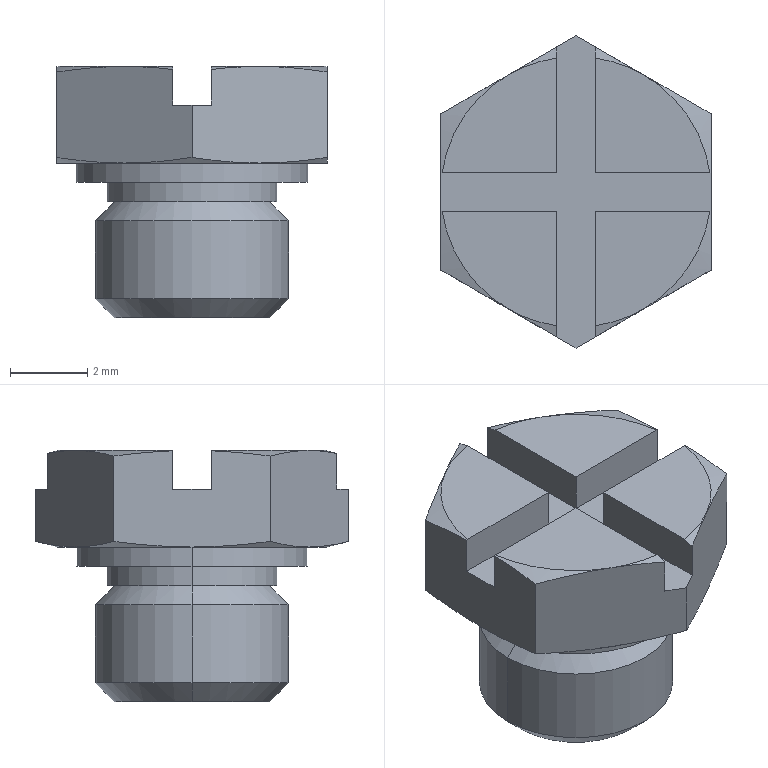Part | SolidWorks | features BaseBody 1 | 1 solid | 47 faces | box 7 x 8.083 x 6.5 mm | volume 169.1 mm3 | plane 23 | cone 18 | cylinder 6 | commonest cylinder face diameters 4.4 x2 5 x2 6 x2
STEP:
#1=CARTESIAN_POINT('',(2.5,0.,-3.01));
#2=VERTEX_POINT('',#1);
#3=CARTESIAN_POINT('',(-2.5,0.,-3.01));
#4=VERTEX_POINT('',#3);
#5=CARTESIAN_POINT('',(0.,0.,-3.01));
#6=DIRECTION('',(0.,0.,1.));
#7=DIRECTION('',(1.,0.,0.));
#8=AXIS2_PLACEMENT_3D('',#5,#6,#7);
#9=CIRCLE('',#8,2.5);
#10=EDGE_CURVE('',#2,#4,#9,.T.);
#11=ORIENTED_EDGE('',*,*,#10,.T.);
#12=CARTESIAN_POINT('',(-2.5,0.,-0.9905));
#13=VERTEX_POINT('',#12);
#14=CARTESIAN_POINT('',(-2.5,0.,-3.5));
#15=DIRECTION('',(0.,0.,1.));
#16=VECTOR('',#15,1000.);
#17=LINE('',#14,#16);
#18=EDGE_CURVE('',#4,#13,#17,.T.);
#19=ORIENTED_EDGE('',*,*,#18,.T.);
#20=CARTESIAN_POINT('',(2.5,0.,-0.9905));
#21=VERTEX_POINT('',#20);
#22=CARTESIAN_POINT('',(0.,0.,-0.9905));
#23=DIRECTION('',(0.,0.,-1.));
#24=DIRECTION('',(1.,0.,0.));
#25=AXIS2_PLACEMENT_3D('',#22,#23,#24);
#26=CIRCLE('',#25,2.5);
#27=EDGE_CURVE('',#13,#21,#26,.T.);
#28=ORIENTED_EDGE('',*,*,#27,.T.);
#29=CARTESIAN_POINT('',(2.5,0.,-3.5));
#30=DIRECTION('',(0.,0.,1.));
#31=VECTOR('',#30,1000.);
#32=LINE('',#29,#31);
#33=EDGE_CURVE('',#2,#21,#32,.T.);
#34=ORIENTED_EDGE('',*,*,#33,.F.);
#35=EDGE_LOOP('',(#11,#19,#28,#34));
#36=FACE_OUTER_BOUND('',#35,.T.);
#37=CARTESIAN_POINT('',(0.,0.,-3.5));
#38=DIRECTION('',(0.,0.,1.));
#39=DIRECTION('',(1.,0.,0.));
#40=AXIS2_PLACEMENT_3D('',#37,#38,#39);
#41=CYLINDRICAL_SURFACE('',#40,2.5);
#42=ADVANCED_FACE('',(#36),#41,.T.);
#43=CARTESIAN_POINT('',(-2.009,0.,-0.5));
#44=VERTEX_POINT('',#43);
#45=CARTESIAN_POINT('',(2.009,0.,-0.5));
#46=VERTEX_POINT('',#45);
#47=CARTESIAN_POINT('',(0.,0.,-0.5));
#48=DIRECTION('',(0.,0.,-1.));
#49=DIRECTION('',(-1.,0.,0.));
#50=AXIS2_PLACEMENT_3D('',#47,#48,#49);
#51=CIRCLE('',#50,2.009);
#52=EDGE_CURVE('',#44,#46,#51,.T.);
#53=ORIENTED_EDGE('',*,*,#52,.T.);
#54=CARTESIAN_POINT('',(2.5,0.,-0.9905));
#55=DIRECTION('',(0.7071,0.,-0.7071));
#56=VECTOR('',#55,1000.);
#57=LINE('',#54,#56);
#58=EDGE_CURVE('',#46,#21,#57,.T.);
#59=ORIENTED_EDGE('',*,*,#58,.T.);
#60=ORIENTED_EDGE('',*,*,#27,.F.);
#61=CARTESIAN_POINT('',(-2.5,0.,-0.9905));
#62=DIRECTION('',(-0.7071,0.,-0.7071));
#63=VECTOR('',#62,1000.);
#64=LINE('',#61,#63);
#65=EDGE_CURVE('',#44,#13,#64,.T.);
#66=ORIENTED_EDGE('',*,*,#65,.F.);
#67=EDGE_LOOP('',(#53,#59,#60,#66));
#68=FACE_OUTER_BOUND('',#67,.T.);
#69=CARTESIAN_POINT('',(0.,0.,-0.9905));
#70=DIRECTION('',(0.,0.,-1.));
#71=DIRECTION('',(-1.,0.,0.));
#72=AXIS2_PLACEMENT_3D('',#69,#70,#71);
#73=CONICAL_SURFACE('',#72,2.5,0.7854);
#74=ADVANCED_FACE('',(#68),#73,.T.);
#75=CARTESIAN_POINT('',(2.009,0.,-3.5));
#76=VERTEX_POINT('',#75);
#77=CARTESIAN_POINT('',(-2.009,0.,-3.5));
#78=VERTEX_POINT('',#77);
#79=CARTESIAN_POINT('',(0.,0.,-3.5));
#80=DIRECTION('',(0.,0.,1.));
#81=DIRECTION('',(1.,0.,0.));
#82=AXIS2_PLACEMENT_3D('',#79,#80,#81);
#83=CIRCLE('',#82,2.009);
#84=EDGE_CURVE('',#76,#78,#83,.T.);
#85=ORIENTED_EDGE('',*,*,#84,.T.);
#86=CARTESIAN_POINT('',(-2.5,0.,-3.01));
#87=DIRECTION('',(-0.7071,0.,0.7071));
#88=VECTOR('',#87,1000.);
#89=LINE('',#86,#88);
#90=EDGE_CURVE('',#78,#4,#89,.T.);
#91=ORIENTED_EDGE('',*,*,#90,.T.);
#92=ORIENTED_EDGE('',*,*,#10,.F.);
#93=CARTESIAN_POINT('',(2.5,0.,-3.01));
#94=DIRECTION('',(0.7071,0.,0.7071));
#95=VECTOR('',#94,1000.);
#96=LINE('',#93,#95);
#97=EDGE_CURVE('',#76,#2,#96,.T.);
#98=ORIENTED_EDGE('',*,*,#97,.F.);
#99=EDGE_LOOP('',(#85,#91,#92,#98));
#100=FACE_OUTER_BOUND('',#99,.T.);
#101=CARTESIAN_POINT('',(0.,0.,-3.01));
#102=DIRECTION('',(0.,0.,1.));
#103=DIRECTION('',(1.,0.,0.));
#104=AXIS2_PLACEMENT_3D('',#101,#102,#103);
#105=CONICAL_SURFACE('',#104,2.5,0.7854);
#106=ADVANCED_FACE('',(#100),#105,.T.);
#107=CARTESIAN_POINT('',(2.2,0.,-0.5));
#108=VERTEX_POINT('',#107);
#109=CARTESIAN_POINT('',(-2.2,0.,-0.5));
#110=VERTEX_POINT('',#109);
#111=CARTESIAN_POINT('',(0.,0.,-0.5));
#112=DIRECTION('',(0.,0.,1.));
#113=DIRECTION('',(1.,0.,0.));
#114=AXIS2_PLACEMENT_3D('',#111,#112,#113);
#115=CIRCLE('',#114,2.2);
#116=EDGE_CURVE('',#108,#110,#115,.T.);
#117=ORIENTED_EDGE('',*,*,#116,.T.);
#118=CARTESIAN_POINT('',(-2.2,0.,0.));
#119=VERTEX_POINT('',#118);
#120=CARTESIAN_POINT('',(-2.2,0.,-3.5));
#121=DIRECTION('',(0.,0.,1.));
#122=VECTOR('',#121,1000.);
#123=LINE('',#120,#122);
#124=EDGE_CURVE('',#110,#119,#123,.T.);
#125=ORIENTED_EDGE('',*,*,#124,.T.);
#126=CARTESIAN_POINT('',(2.2,0.,0.));
#127=VERTEX_POINT('',#126);
#128=CARTESIAN_POINT('',(0.,0.,0.));
#129=DIRECTION('',(0.,0.,-1.));
#130=DIRECTION('',(1.,0.,0.));
#131=AXIS2_PLACEMENT_3D('',#128,#129,#130);
#132=CIRCLE('',#131,2.2);
#133=EDGE_CURVE('',#119,#127,#132,.T.);
#134=ORIENTED_EDGE('',*,*,#133,.T.);
#135=CARTESIAN_POINT('',(2.2,0.,-3.5));
#136=DIRECTION('',(0.,0.,1.));
#137=VECTOR('',#136,1000.);
#138=LINE('',#135,#137);
#139=EDGE_CURVE('',#108,#127,#138,.T.);
#140=ORIENTED_EDGE('',*,*,#139,.F.);
#141=EDGE_LOOP('',(#117,#125,#134,#140));
#142=FACE_OUTER_BOUND('',#141,.T.);
#143=CARTESIAN_POINT('',(0.,0.,-3.5));
#144=DIRECTION('',(0.,0.,1.));
#145=DIRECTION('',(1.,0.,0.));
#146=AXIS2_PLACEMENT_3D('',#143,#144,#145);
#147=CYLINDRICAL_SURFACE('',#146,2.2);
#148=ADVANCED_FACE('',(#142),#147,.T.);
#149=CARTESIAN_POINT('',(3.,0.,0.));
#150=VERTEX_POINT('',#149);
#151=CARTESIAN_POINT('',(-3.,0.,0.));
#152=VERTEX_POINT('',#151);
#153=CARTESIAN_POINT('',(0.,0.,0.));
#154=DIRECTION('',(0.,0.,1.));
#155=DIRECTION('',(1.,0.,0.));
#156=AXIS2_PLACEMENT_3D('',#153,#154,#155);
#157=CIRCLE('',#156,3.);
#158=EDGE_CURVE('',#150,#152,#157,.T.);
#159=ORIENTED_EDGE('',*,*,#158,.T.);
#160=CARTESIAN_POINT('',(-3.,0.,0.5));
#161=VERTEX_POINT('',#160);
#162=CARTESIAN_POINT('',(-3.,0.,-3.5));
#163=DIRECTION('',(0.,0.,1.));
#164=VECTOR('',#163,1000.);
#165=LINE('',#162,#164);
#166=EDGE_CURVE('',#152,#161,#165,.T.);
#167=ORIENTED_EDGE('',*,*,#166,.T.);
#168=CARTESIAN_POINT('',(3.,0.,0.5));
#169=VERTEX_POINT('',#168);
#170=CARTESIAN_POINT('',(0.,0.,0.5));
#171=DIRECTION('',(0.,0.,-1.));
#172=DIRECTION('',(1.,0.,0.));
#173=AXIS2_PLACEMENT_3D('',#170,#171,#172);
#174=CIRCLE('',#173,3.);
#175=EDGE_CURVE('',#161,#169,#174,.T.);
#176=ORIENTED_EDGE('',*,*,#175,.T.);
#177=CARTESIAN_POINT('',(3.,0.,-3.5));
#178=DIRECTION('',(0.,0.,1.));
#179=VECTOR('',#178,1000.);
#180=LINE('',#177,#179);
#181=EDGE_CURVE('',#150,#169,#180,.T.);
#182=ORIENTED_EDGE('',*,*,#181,.F.);
#183=EDGE_LOOP('',(#159,#167,#176,#182));
#184=FACE_OUTER_BOUND('',#183,.T.);
#185=CARTESIAN_POINT('',(0.,0.,-3.5));
#186=DIRECTION('',(0.,0.,1.));
#187=DIRECTION('',(1.,0.,0.));
#188=AXIS2_PLACEMENT_3D('',#185,#186,#187);
#189=CYLINDRICAL_SURFACE('',#188,3.);
#190=ADVANCED_FACE('',(#184),#189,.T.);
#191=ORIENTED_EDGE('',*,*,#18,.F.);
#192=CARTESIAN_POINT('',(0.,0.,-3.01));
#193=DIRECTION('',(0.,0.,1.));
#194=DIRECTION('',(1.,0.,0.));
#195=AXIS2_PLACEMENT_3D('',#192,#193,#194);
#196=CIRCLE('',#195,2.5);
#197=EDGE_CURVE('',#4,#2,#196,.T.);
#198=ORIENTED_EDGE('',*,*,#197,.T.);
#199=ORIENTED_EDGE('',*,*,#33,.T.);
#200=CARTESIAN_POINT('',(0.,0.,-0.9905));
#201=DIRECTION('',(0.,0.,-1.));
#202=DIRECTION('',(1.,0.,0.));
#203=AXIS2_PLACEMENT_3D('',#200,#201,#202);
#204=CIRCLE('',#203,2.5);
#205=EDGE_CURVE('',#21,#13,#204,.T.);
#206=ORIENTED_EDGE('',*,*,#205,.T.);
#207=EDGE_LOOP('',(#191,#198,#199,#206));
#208=FACE_OUTER_BOUND('',#207,.T.);
#209=CARTESIAN_POINT('',(0.,0.,-3.5));
#210=DIRECTION('',(0.,0.,1.));
#211=DIRECTION('',(1.,0.,0.));
#212=AXIS2_PLACEMENT_3D('',#209,#210,#211);
#213=CYLINDRICAL_SURFACE('',#212,2.5);
#214=ADVANCED_FACE('',(#208),#213,.T.);
#215=ORIENTED_EDGE('',*,*,#58,.F.);
#216=CARTESIAN_POINT('',(0.,0.,-0.5));
#217=DIRECTION('',(0.,0.,-1.));
#218=DIRECTION('',(-1.,0.,0.));
#219=AXIS2_PLACEMENT_3D('',#216,#217,#218);
#220=CIRCLE('',#219,2.009);
#221=EDGE_CURVE('',#46,#44,#220,.T.);
#222=ORIENTED_EDGE('',*,*,#221,.T.);
#223=ORIENTED_EDGE('',*,*,#65,.T.);
#224=ORIENTED_EDGE('',*,*,#205,.F.);
#225=EDGE_LOOP('',(#215,#222,#223,#224));
#226=FACE_OUTER_BOUND('',#225,.T.);
#227=CARTESIAN_POINT('',(0.,0.,-0.9905));
#228=DIRECTION('',(0.,0.,-1.));
#229=DIRECTION('',(-1.,0.,0.));
#230=AXIS2_PLACEMENT_3D('',#227,#228,#229);
#231=CONICAL_SURFACE('',#230,2.5,0.7854);
#232=ADVANCED_FACE('',(#226),#231,.T.);
#233=ORIENTED_EDGE('',*,*,#90,.F.);
#234=CARTESIAN_POINT('',(0.,0.,-3.5));
#235=DIRECTION('',(0.,0.,1.));
#236=DIRECTION('',(1.,0.,0.));
#237=AXIS2_PLACEMENT_3D('',#234,#235,#236);
#238=CIRCLE('',#237,2.009);
#239=EDGE_CURVE('',#78,#76,#238,.T.);
#240=ORIENTED_EDGE('',*,*,#239,.T.);
#241=ORIENTED_EDGE('',*,*,#97,.T.);
#242=ORIENTED_EDGE('',*,*,#197,.F.);
#243=EDGE_LOOP('',(#233,#240,#241,#242));
#244=FACE_OUTER_BOUND('',#243,.T.);
#245=CARTESIAN_POINT('',(0.,0.,-3.01));
#246=DIRECTION('',(0.,0.,1.));
#247=DIRECTION('',(1.,0.,0.));
#248=AXIS2_PLACEMENT_3D('',#245,#246,#247);
#249=CONICAL_SURFACE('',#248,2.5,0.7854);
#250=ADVANCED_FACE('',(#244),#249,.T.);
#251=ORIENTED_EDGE('',*,*,#52,.F.);
#252=ORIENTED_EDGE('',*,*,#221,.F.);
#253=EDGE_LOOP('',(#251,#252));
#254=FACE_BOUND('',#253,.T.);
#255=ORIENTED_EDGE('',*,*,#116,.F.);
#256=CARTESIAN_POINT('',(0.,0.,-0.5));
#257=DIRECTION('',(0.,0.,1.));
#258=DIRECTION('',(1.,0.,0.));
#259=AXIS2_PLACEMENT_3D('',#256,#257,#258);
#260=CIRCLE('',#259,2.2);
#261=EDGE_CURVE('',#110,#108,#260,.T.);
#262=ORIENTED_EDGE('',*,*,#261,.F.);
#263=EDGE_LOOP('',(#255,#262));
#264=FACE_OUTER_BOUND('',#263,.T.);
#265=CARTESIAN_POINT('',(0.,2.2,-0.5));
#266=DIRECTION('',(0.,0.,1.));
#267=DIRECTION('',(1.,0.,0.));
#268=AXIS2_PLACEMENT_3D('',#265,#266,#267);
#269=PLANE('',#268);
#270=ADVANCED_FACE('',(#254,#264),#269,.F.);
#271=ORIENTED_EDGE('',*,*,#84,.F.);
#272=ORIENTED_EDGE('',*,*,#239,.F.);
#273=EDGE_LOOP('',(#271,#272));
#274=FACE_OUTER_BOUND('',#273,.T.);
#275=CARTESIAN_POINT('',(0.,2.01,-3.5));
#276=DIRECTION('',(0.,0.,1.));
#277=DIRECTION('',(1.,0.,0.));
#278=AXIS2_PLACEMENT_3D('',#275,#276,#277);
#279=PLANE('',#278);
#280=ADVANCED_FACE('',(#274),#279,.F.);
#281=ORIENTED_EDGE('',*,*,#124,.F.);
#282=ORIENTED_EDGE('',*,*,#261,.T.);
#283=ORIENTED_EDGE('',*,*,#139,.T.);
#284=CARTESIAN_POINT('',(0.,0.,0.));
#285=DIRECTION('',(0.,0.,-1.));
#286=DIRECTION('',(1.,0.,0.));
#287=AXIS2_PLACEMENT_3D('',#284,#285,#286);
#288=CIRCLE('',#287,2.2);
#289=EDGE_CURVE('',#127,#119,#288,.T.);
#290=ORIENTED_EDGE('',*,*,#289,.T.);
#291=EDGE_LOOP('',(#281,#282,#283,#290));
#292=FACE_OUTER_BOUND('',#291,.T.);
#293=CARTESIAN_POINT('',(0.,0.,-3.5));
#294=DIRECTION('',(0.,0.,1.));
#295=DIRECTION('',(1.,0.,0.));
#296=AXIS2_PLACEMENT_3D('',#293,#294,#295);
#297=CYLINDRICAL_SURFACE('',#296,2.2);
#298=ADVANCED_FACE('',(#292),#297,.T.);
#299=ORIENTED_EDGE('',*,*,#289,.F.);
#300=ORIENTED_EDGE('',*,*,#133,.F.);
#301=EDGE_LOOP('',(#299,#300));
#302=FACE_BOUND('',#301,.T.);
#303=ORIENTED_EDGE('',*,*,#158,.F.);
#304=CARTESIAN_POINT('',(0.,0.,0.));
#305=DIRECTION('',(0.,0.,1.));
#306=DIRECTION('',(1.,0.,0.));
#307=AXIS2_PLACEMENT_3D('',#304,#305,#306);
#308=CIRCLE('',#307,3.);
#309=EDGE_CURVE('',#152,#150,#308,.T.);
#310=ORIENTED_EDGE('',*,*,#309,.F.);
#311=EDGE_LOOP('',(#303,#310));
#312=FACE_OUTER_BOUND('',#311,.T.);
#313=CARTESIAN_POINT('',(0.,3.,0.));
#314=DIRECTION('',(0.,0.,1.));
#315=DIRECTION('',(1.,0.,0.));
#316=AXIS2_PLACEMENT_3D('',#313,#314,#315);
#317=PLANE('',#316);
#318=ADVANCED_FACE('',(#302,#312),#317,.F.);
#319=ORIENTED_EDGE('',*,*,#166,.F.);
#320=ORIENTED_EDGE('',*,*,#309,.T.);
#321=ORIENTED_EDGE('',*,*,#181,.T.);
#322=CARTESIAN_POINT('',(0.,0.,0.5));
#323=DIRECTION('',(0.,0.,-1.));
#324=DIRECTION('',(1.,0.,0.));
#325=AXIS2_PLACEMENT_3D('',#322,#323,#324);
#326=CIRCLE('',#325,3.);
#327=EDGE_CURVE('',#169,#161,#326,.T.);
#328=ORIENTED_EDGE('',*,*,#327,.T.);
#329=EDGE_LOOP('',(#319,#320,#321,#328));
#330=FACE_OUTER_BOUND('',#329,.T.);
#331=CARTESIAN_POINT('',(0.,0.,-3.5));
#332=DIRECTION('',(0.,0.,1.));
#333=DIRECTION('',(1.,0.,0.));
#334=AXIS2_PLACEMENT_3D('',#331,#332,#333);
#335=CYLINDRICAL_SURFACE('',#334,3.);
#336=ADVANCED_FACE('',(#330),#335,.T.);
#337=ORIENTED_EDGE('',*,*,#327,.F.);
#338=ORIENTED_EDGE('',*,*,#175,.F.);
#339=EDGE_LOOP('',(#337,#338));
#340=FACE_BOUND('',#339,.T.);
#341=CARTESIAN_POINT('',(3.5,0.,0.5));
#342=VERTEX_POINT('',#341);
#343=CARTESIAN_POINT('',(1.75,3.031,0.5));
#344=VERTEX_POINT('',#343);
#345=CARTESIAN_POINT('',(0.,0.,0.5));
#346=DIRECTION('',(0.,0.,1.));
#347=DIRECTION('',(1.,0.,0.));
#348=AXIS2_PLACEMENT_3D('',#345,#346,#347);
#349=CIRCLE('',#348,3.5);
#350=EDGE_CURVE('',#342,#344,#349,.T.);
#351=ORIENTED_EDGE('',*,*,#350,.F.);
#352=CARTESIAN_POINT('',(1.75,-3.031,0.5));
#353=VERTEX_POINT('',#352);
#354=CARTESIAN_POINT('',(0.,0.,0.5));
#355=DIRECTION('',(0.,0.,1.));
#356=DIRECTION('',(1.,0.,0.));
#357=AXIS2_PLACEMENT_3D('',#354,#355,#356);
#358=CIRCLE('',#357,3.5);
#359=EDGE_CURVE('',#353,#342,#358,.T.);
#360=ORIENTED_EDGE('',*,*,#359,.F.);
#361=CARTESIAN_POINT('',(-1.75,-3.031,0.5));
#362=VERTEX_POINT('',#361);
#363=CARTESIAN_POINT('',(0.,0.,0.5));
#364=DIRECTION('',(0.,0.,1.));
#365=DIRECTION('',(1.,0.,0.));
#366=AXIS2_PLACEMENT_3D('',#363,#364,#365);
#367=CIRCLE('',#366,3.5);
#368=EDGE_CURVE('',#362,#353,#367,.T.);
#369=ORIENTED_EDGE('',*,*,#368,.F.);
#370=CARTESIAN_POINT('',(-3.5,0.,0.5));
#371=VERTEX_POINT('',#370);
#372=CARTESIAN_POINT('',(0.,0.,0.5));
#373=DIRECTION('',(0.,0.,1.));
#374=DIRECTION('',(1.,0.,0.));
#375=AXIS2_PLACEMENT_3D('',#372,#373,#374);
#376=CIRCLE('',#375,3.5);
#377=EDGE_CURVE('',#371,#362,#376,.T.);
#378=ORIENTED_EDGE('',*,*,#377,.F.);
#379=CARTESIAN_POINT('',(-1.75,3.031,0.5));
#380=VERTEX_POINT('',#379);
#381=CARTESIAN_POINT('',(0.,0.,0.5));
#382=DIRECTION('',(0.,0.,1.));
#383=DIRECTION('',(1.,0.,0.));
#384=AXIS2_PLACEMENT_3D('',#381,#382,#383);
#385=CIRCLE('',#384,3.5);
#386=EDGE_CURVE('',#380,#371,#385,.T.);
#387=ORIENTED_EDGE('',*,*,#386,.F.);
#388=CARTESIAN_POINT('',(0.,0.,0.5));
#389=DIRECTION('',(0.,0.,1.));
#390=DIRECTION('',(1.,0.,0.));
#391=AXIS2_PLACEMENT_3D('',#388,#389,#390);
#392=CIRCLE('',#391,3.5);
#393=EDGE_CURVE('',#344,#380,#392,.T.);
#394=ORIENTED_EDGE('',*,*,#393,.F.);
#395=EDGE_LOOP('',(#351,#360,#369,#378,#387,#394));
#396=FACE_OUTER_BOUND('',#395,.T.);
#397=CARTESIAN_POINT('',(0.,3.5,0.5));
#398=DIRECTION('',(0.,0.,1.));
#399=DIRECTION('',(1.,0.,0.));
#400=AXIS2_PLACEMENT_3D('',#397,#398,#399);
#401=PLANE('',#400);
#402=ADVANCED_FACE('',(#340,#396),#401,.F.);
#403=CARTESIAN_POINT('',(-0.000000057,4.041,0.6451));
#404=VERTEX_POINT('',#403);
#405=CARTESIAN_POINT('',(-0.000000057,4.041,0.6451));
#406=CARTESIAN_POINT('',(0.5808,3.706,0.5552));
#407=CARTESIAN_POINT('',(1.164,3.37,0.5));
#408=CARTESIAN_POINT('',(1.75,3.031,0.5));
#409=B_SPLINE_CURVE_WITH_KNOTS('',3,(#405,#406,#407,#408),.UNSPECIFIED.,.F.,.F.,(4,4),(0.,0.002026),.UNSPECIFIED.);
#410=EDGE_CURVE('',#404,#344,#409,.T.);
#411=ORIENTED_EDGE('',*,*,#410,.T.);
#412=ORIENTED_EDGE('',*,*,#393,.T.);
#413=CARTESIAN_POINT('',(-1.75,3.031,0.5));
#414=CARTESIAN_POINT('',(-1.164,3.37,0.5));
#415=CARTESIAN_POINT('',(-0.5808,3.706,0.5552));
#416=CARTESIAN_POINT('',(-0.000000057,4.041,0.6451));
#417=B_SPLINE_CURVE_WITH_KNOTS('',3,(#413,#414,#415,#416),.UNSPECIFIED.,.F.,.F.,(4,4),(0.,0.002026),.UNSPECIFIED.);
#418=EDGE_CURVE('',#380,#404,#417,.T.);
#419=ORIENTED_EDGE('',*,*,#418,.T.);
#420=EDGE_LOOP('',(#411,#412,#419));
#421=FACE_OUTER_BOUND('',#420,.T.);
#422=CARTESIAN_POINT('',(0.,0.,0.646));
#423=DIRECTION('',(0.,0.,1.));
#424=DIRECTION('',(1.,0.,0.));
#425=AXIS2_PLACEMENT_3D('',#422,#423,#424);
#426=CONICAL_SURFACE('',#425,4.045,1.309);
#427=ADVANCED_FACE('',(#421),#426,.T.);
#428=CARTESIAN_POINT('',(3.5,2.021,0.6451));
#429=VERTEX_POINT('',#428);
#430=CARTESIAN_POINT('',(3.5,2.021,0.6451));
#431=CARTESIAN_POINT('',(3.5,1.35,0.5552));
#432=CARTESIAN_POINT('',(3.5,0.677,0.5));
#433=CARTESIAN_POINT('',(3.5,0.,0.5));
#434=B_SPLINE_CURVE_WITH_KNOTS('',3,(#430,#431,#432,#433),.UNSPECIFIED.,.F.,.F.,(4,4),(0.,0.002026),.UNSPECIFIED.);
#435=EDGE_CURVE('',#429,#342,#434,.T.);
#436=ORIENTED_EDGE('',*,*,#435,.T.);
#437=ORIENTED_EDGE('',*,*,#350,.T.);
#438=CARTESIAN_POINT('',(1.75,3.031,0.5));
#439=CARTESIAN_POINT('',(2.336,2.693,0.5));
#440=CARTESIAN_POINT('',(2.919,2.356,0.5552));
#441=CARTESIAN_POINT('',(3.5,2.021,0.6451));
#442=B_SPLINE_CURVE_WITH_KNOTS('',3,(#438,#439,#440,#441),.UNSPECIFIED.,.F.,.F.,(4,4),(0.,0.002026),.UNSPECIFIED.);
#443=EDGE_CURVE('',#344,#429,#442,.T.);
#444=ORIENTED_EDGE('',*,*,#443,.T.);
#445=EDGE_LOOP('',(#436,#437,#444));
#446=FACE_OUTER_BOUND('',#445,.T.);
#447=CARTESIAN_POINT('',(0.,0.,0.646));
#448=DIRECTION('',(0.,0.,1.));
#449=DIRECTION('',(1.,0.,0.));
#450=AXIS2_PLACEMENT_3D('',#447,#448,#449);
#451=CONICAL_SURFACE('',#450,4.045,1.309);
#452=ADVANCED_FACE('',(#446),#451,.T.);
#453=CARTESIAN_POINT('',(3.5,-2.021,0.6451));
#454=VERTEX_POINT('',#453);
#455=CARTESIAN_POINT('',(3.5,-2.021,0.6451));
#456=CARTESIAN_POINT('',(2.919,-2.356,0.5552));
#457=CARTESIAN_POINT('',(2.336,-2.693,0.5));
#458=CARTESIAN_POINT('',(1.75,-3.031,0.5));
#459=B_SPLINE_CURVE_WITH_KNOTS('',3,(#455,#456,#457,#458),.UNSPECIFIED.,.F.,.F.,(4,4),(0.,0.002026),.UNSPECIFIED.);
#460=EDGE_CURVE('',#454,#353,#459,.T.);
#461=ORIENTED_EDGE('',*,*,#460,.T.);
#462=ORIENTED_EDGE('',*,*,#359,.T.);
#463=CARTESIAN_POINT('',(3.5,0.,0.5));
#464=CARTESIAN_POINT('',(3.5,-0.677,0.5));
#465=CARTESIAN_POINT('',(3.5,-1.35,0.5552));
#466=CARTESIAN_POINT('',(3.5,-2.021,0.6451));
#467=B_SPLINE_CURVE_WITH_KNOTS('',3,(#463,#464,#465,#466),.UNSPECIFIED.,.F.,.F.,(4,4),(0.,0.002026),.UNSPECIFIED.);
#468=EDGE_CURVE('',#342,#454,#467,.T.);
#469=ORIENTED_EDGE('',*,*,#468,.T.);
#470=EDGE_LOOP('',(#461,#462,#469));
#471=FACE_OUTER_BOUND('',#470,.T.);
#472=CARTESIAN_POINT('',(0.,0.,0.646));
#473=DIRECTION('',(0.,0.,1.));
#474=DIRECTION('',(1.,0.,0.));
#475=AXIS2_PLACEMENT_3D('',#472,#473,#474);
#476=CONICAL_SURFACE('',#475,4.045,1.309);
#477=ADVANCED_FACE('',(#471),#476,.T.);
#478=CARTESIAN_POINT('',(0.000000064,-4.041,0.6451));
#479=VERTEX_POINT('',#478);
#480=CARTESIAN_POINT('',(0.000000064,-4.041,0.6451));
#481=CARTESIAN_POINT('',(-0.5808,-3.706,0.5552));
#482=CARTESIAN_POINT('',(-1.164,-3.37,0.5));
#483=CARTESIAN_POINT('',(-1.75,-3.031,0.5));
#484=B_SPLINE_CURVE_WITH_KNOTS('',3,(#480,#481,#482,#483),.UNSPECIFIED.,.F.,.F.,(4,4),(0.,0.002026),.UNSPECIFIED.);
#485=EDGE_CURVE('',#479,#362,#484,.T.);
#486=ORIENTED_EDGE('',*,*,#485,.T.);
#487=ORIENTED_EDGE('',*,*,#368,.T.);
#488=CARTESIAN_POINT('',(1.75,-3.031,0.5));
#489=CARTESIAN_POINT('',(1.164,-3.37,0.5));
#490=CARTESIAN_POINT('',(0.5808,-3.706,0.5552));
#491=CARTESIAN_POINT('',(0.000000064,-4.041,0.6451));
#492=B_SPLINE_CURVE_WITH_KNOTS('',3,(#488,#489,#490,#491),.UNSPECIFIED.,.F.,.F.,(4,4),(0.,0.002026),.UNSPECIFIED.);
#493=EDGE_CURVE('',#353,#479,#492,.T.);
#494=ORIENTED_EDGE('',*,*,#493,.T.);
#495=EDGE_LOOP('',(#486,#487,#494));
#496=FACE_OUTER_BOUND('',#495,.T.);
#497=CARTESIAN_POINT('',(0.,0.,0.646));
#498=DIRECTION('',(0.,0.,1.));
#499=DIRECTION('',(1.,0.,0.));
#500=AXIS2_PLACEMENT_3D('',#497,#498,#499);
#501=CONICAL_SURFACE('',#500,4.045,1.309);
#502=ADVANCED_FACE('',(#496),#501,.T.);
#503=ORIENTED_EDGE('',*,*,#377,.T.);
#504=CARTESIAN_POINT('',(-3.5,-2.021,0.6451));
#505=VERTEX_POINT('',#504);
#506=CARTESIAN_POINT('',(-1.75,-3.031,0.5));
#507=CARTESIAN_POINT('',(-2.336,-2.693,0.5));
#508=CARTESIAN_POINT('',(-2.919,-2.356,0.5552));
#509=CARTESIAN_POINT('',(-3.5,-2.021,0.6451));
#510=B_SPLINE_CURVE_WITH_KNOTS('',3,(#506,#507,#508,#509),.UNSPECIFIED.,.F.,.F.,(4,4),(0.,0.002026),.UNSPECIFIED.);
#511=EDGE_CURVE('',#362,#505,#510,.T.);
#512=ORIENTED_EDGE('',*,*,#511,.T.);
#513=CARTESIAN_POINT('',(-3.5,-2.021,0.6451));
#514=CARTESIAN_POINT('',(-3.5,-1.35,0.5552));
#515=CARTESIAN_POINT('',(-3.5,-0.677,0.5));
#516=CARTESIAN_POINT('',(-3.5,0.,0.5));
#517=B_SPLINE_CURVE_WITH_KNOTS('',3,(#513,#514,#515,#516),.UNSPECIFIED.,.F.,.F.,(4,4),(0.,0.002026),.UNSPECIFIED.);
#518=EDGE_CURVE('',#505,#371,#517,.T.);
#519=ORIENTED_EDGE('',*,*,#518,.T.);
#520=EDGE_LOOP('',(#503,#512,#519));
#521=FACE_OUTER_BOUND('',#520,.T.);
#522=CARTESIAN_POINT('',(0.,0.,0.646));
#523=DIRECTION('',(0.,0.,1.));
#524=DIRECTION('',(1.,0.,0.));
#525=AXIS2_PLACEMENT_3D('',#522,#523,#524);
#526=CONICAL_SURFACE('',#525,4.045,1.309);
#527=ADVANCED_FACE('',(#521),#526,.T.);
#528=CARTESIAN_POINT('',(-3.5,2.021,0.6451));
#529=VERTEX_POINT('',#528);
#530=CARTESIAN_POINT('',(-3.5,2.021,0.6451));
#531=CARTESIAN_POINT('',(-2.919,2.356,0.5552));
#532=CARTESIAN_POINT('',(-2.336,2.693,0.5));
#533=CARTESIAN_POINT('',(-1.75,3.031,0.5));
#534=B_SPLINE_CURVE_WITH_KNOTS('',3,(#530,#531,#532,#533),.UNSPECIFIED.,.F.,.F.,(4,4),(0.,0.002026),.UNSPECIFIED.);
#535=EDGE_CURVE('',#529,#380,#534,.T.);
#536=ORIENTED_EDGE('',*,*,#535,.T.);
#537=ORIENTED_EDGE('',*,*,#386,.T.);
#538=CARTESIAN_POINT('',(-3.5,0.,0.5));
#539=CARTESIAN_POINT('',(-3.5,0.677,0.5));
#540=CARTESIAN_POINT('',(-3.5,1.35,0.5552));
#541=CARTESIAN_POINT('',(-3.5,2.021,0.6451));
#542=B_SPLINE_CURVE_WITH_KNOTS('',3,(#538,#539,#540,#541),.UNSPECIFIED.,.F.,.F.,(4,4),(0.,0.002026),.UNSPECIFIED.);
#543=EDGE_CURVE('',#371,#529,#542,.T.);
#544=ORIENTED_EDGE('',*,*,#543,.T.);
#545=EDGE_LOOP('',(#536,#537,#544));
#546=FACE_OUTER_BOUND('',#545,.T.);
#547=CARTESIAN_POINT('',(0.,0.,0.646));
#548=DIRECTION('',(0.,0.,1.));
#549=DIRECTION('',(1.,0.,0.));
#550=AXIS2_PLACEMENT_3D('',#547,#548,#549);
#551=CONICAL_SURFACE('',#550,4.045,1.309);
#552=ADVANCED_FACE('',(#546),#551,.T.);
#553=CARTESIAN_POINT('',(1.75,3.031,3.));
#554=VERTEX_POINT('',#553);
#555=CARTESIAN_POINT('',(0.5,3.753,2.923));
#556=VERTEX_POINT('',#555);
#557=CARTESIAN_POINT('',(1.75,3.031,3.));
#558=CARTESIAN_POINT('',(1.332,3.272,3.));
#559=CARTESIAN_POINT('',(0.9156,3.513,2.972));
#560=CARTESIAN_POINT('',(0.5,3.753,2.923));
#561=B_SPLINE_CURVE_WITH_KNOTS('',3,(#557,#558,#559,#560),.UNSPECIFIED.,.F.,.F.,(4,4),(0.,0.001445),.UNSPECIFIED.);
#562=EDGE_CURVE('',#554,#556,#561,.T.);
#563=ORIENTED_EDGE('',*,*,#562,.F.);
#564=CARTESIAN_POINT('',(3.5,2.021,2.855));
#565=VERTEX_POINT('',#564);
#566=CARTESIAN_POINT('',(3.5,2.021,2.855));
#567=CARTESIAN_POINT('',(2.919,2.356,2.945));
#568=CARTESIAN_POINT('',(2.336,2.693,3.));
#569=CARTESIAN_POINT('',(1.75,3.031,3.));
#570=B_SPLINE_CURVE_WITH_KNOTS('',3,(#566,#567,#568,#569),.UNSPECIFIED.,.F.,.F.,(4,4),(0.,0.002026),.UNSPECIFIED.);
#571=EDGE_CURVE('',#565,#554,#570,.T.);
#572=ORIENTED_EDGE('',*,*,#571,.F.);
#573=CARTESIAN_POINT('',(3.5,2.021,3.));
#574=DIRECTION('',(0.,0.,1.));
#575=VECTOR('',#574,1000.);
#576=LINE('',#573,#575);
#577=EDGE_CURVE('',#429,#565,#576,.T.);
#578=ORIENTED_EDGE('',*,*,#577,.F.);
#579=ORIENTED_EDGE('',*,*,#443,.F.);
#580=ORIENTED_EDGE('',*,*,#410,.F.);
#581=CARTESIAN_POINT('',(0.,4.041,2.));
#582=VERTEX_POINT('',#581);
#583=CARTESIAN_POINT('',(0.,4.041,3.));
#584=DIRECTION('',(0.,0.,-1.));
#585=VECTOR('',#584,1000.);
#586=LINE('',#583,#585);
#587=EDGE_CURVE('',#582,#404,#586,.T.);
#588=ORIENTED_EDGE('',*,*,#587,.F.);
#589=CARTESIAN_POINT('',(0.5,3.753,2.));
#590=VERTEX_POINT('',#589);
#591=CARTESIAN_POINT('',(0.5,3.753,2.));
#592=DIRECTION('',(-0.866,0.5,0.));
#593=VECTOR('',#592,1000.);
#594=LINE('',#591,#593);
#595=EDGE_CURVE('',#590,#582,#594,.T.);
#596=ORIENTED_EDGE('',*,*,#595,.F.);
#597=CARTESIAN_POINT('',(0.5,3.753,2.));
#598=DIRECTION('',(0.,0.,1.));
#599=VECTOR('',#598,1000.);
#600=LINE('',#597,#599);
#601=EDGE_CURVE('',#590,#556,#600,.T.);
#602=ORIENTED_EDGE('',*,*,#601,.T.);
#603=EDGE_LOOP('',(#563,#572,#578,#579,#580,#588,#596,#602));
#604=FACE_OUTER_BOUND('',#603,.T.);
#605=CARTESIAN_POINT('',(3.5,2.021,3.));
#606=DIRECTION('',(-0.5,-0.866,0.));
#607=DIRECTION('',(0.866,-0.5,0.));
#608=AXIS2_PLACEMENT_3D('',#605,#606,#607);
#609=PLANE('',#608);
#610=ADVANCED_FACE('',(#604),#609,.F.);
#611=CARTESIAN_POINT('',(-0.5,3.753,2.));
#612=VERTEX_POINT('',#611);
#613=CARTESIAN_POINT('',(0.,4.041,2.));
#614=DIRECTION('',(-0.866,-0.5,0.));
#615=VECTOR('',#614,1000.);
#616=LINE('',#613,#615);
#617=EDGE_CURVE('',#582,#612,#616,.T.);
#618=ORIENTED_EDGE('',*,*,#617,.F.);
#619=ORIENTED_EDGE('',*,*,#587,.T.);
#620=ORIENTED_EDGE('',*,*,#418,.F.);
#621=ORIENTED_EDGE('',*,*,#535,.F.);
#622=CARTESIAN_POINT('',(-3.5,2.021,2.855));
#623=VERTEX_POINT('',#622);
#624=CARTESIAN_POINT('',(-3.5,2.021,3.));
#625=DIRECTION('',(0.,0.,-1.));
#626=VECTOR('',#625,1000.);
#627=LINE('',#624,#626);
#628=EDGE_CURVE('',#623,#529,#627,.T.);
#629=ORIENTED_EDGE('',*,*,#628,.F.);
#630=CARTESIAN_POINT('',(-1.75,3.031,3.));
#631=VERTEX_POINT('',#630);
#632=CARTESIAN_POINT('',(-1.75,3.031,3.));
#633=CARTESIAN_POINT('',(-2.336,2.693,3.));
#634=CARTESIAN_POINT('',(-2.919,2.356,2.945));
#635=CARTESIAN_POINT('',(-3.5,2.021,2.855));
#636=B_SPLINE_CURVE_WITH_KNOTS('',3,(#632,#633,#634,#635),.UNSPECIFIED.,.F.,.F.,(4,4),(0.,0.002026),.UNSPECIFIED.);
#637=EDGE_CURVE('',#631,#623,#636,.T.);
#638=ORIENTED_EDGE('',*,*,#637,.F.);
#639=CARTESIAN_POINT('',(-0.5,3.753,2.923));
#640=VERTEX_POINT('',#639);
#641=CARTESIAN_POINT('',(-0.5,3.753,2.923));
#642=CARTESIAN_POINT('',(-0.9156,3.513,2.972));
#643=CARTESIAN_POINT('',(-1.332,3.272,3.));
#644=CARTESIAN_POINT('',(-1.75,3.031,3.));
#645=B_SPLINE_CURVE_WITH_KNOTS('',3,(#641,#642,#643,#644),.UNSPECIFIED.,.F.,.F.,(4,4),(0.,0.001445),.UNSPECIFIED.);
#646=EDGE_CURVE('',#640,#631,#645,.T.);
#647=ORIENTED_EDGE('',*,*,#646,.F.);
#648=CARTESIAN_POINT('',(-0.5,3.753,2.));
#649=DIRECTION('',(0.,0.,-1.));
#650=VECTOR('',#649,1000.);
#651=LINE('',#648,#650);
#652=EDGE_CURVE('',#640,#612,#651,.T.);
#653=ORIENTED_EDGE('',*,*,#652,.T.);
#654=EDGE_LOOP('',(#618,#619,#620,#621,#629,#638,#647,#653));
#655=FACE_OUTER_BOUND('',#654,.T.);
#656=CARTESIAN_POINT('',(0.,4.041,3.));
#657=DIRECTION('',(0.5,-0.866,0.));
#658=DIRECTION('',(0.866,0.5,0.));
#659=AXIS2_PLACEMENT_3D('',#656,#657,#658);
#660=PLANE('',#659);
#661=ADVANCED_FACE('',(#655),#660,.F.);
#662=CARTESIAN_POINT('',(3.5,-2.021,2.855));
#663=VERTEX_POINT('',#662);
#664=CARTESIAN_POINT('',(3.5,-0.5,2.99));
#665=VERTEX_POINT('',#664);
#666=CARTESIAN_POINT('',(3.5,-2.021,2.855));
#667=CARTESIAN_POINT('',(3.5,-1.516,2.923));
#668=CARTESIAN_POINT('',(3.5,-1.009,2.971));
#669=CARTESIAN_POINT('',(3.5,-0.5,2.99));
#670=B_SPLINE_CURVE_WITH_KNOTS('',3,(#666,#667,#668,#669),.UNSPECIFIED.,.F.,.F.,(4,4),(0.,0.001527),.UNSPECIFIED.);
#671=EDGE_CURVE('',#663,#665,#670,.T.);
#672=ORIENTED_EDGE('',*,*,#671,.F.);
#673=CARTESIAN_POINT('',(3.5,-2.021,3.));
#674=DIRECTION('',(0.,0.,1.));
#675=VECTOR('',#674,1000.);
#676=LINE('',#673,#675);
#677=EDGE_CURVE('',#454,#663,#676,.T.);
#678=ORIENTED_EDGE('',*,*,#677,.F.);
#679=ORIENTED_EDGE('',*,*,#468,.F.);
#680=ORIENTED_EDGE('',*,*,#435,.F.);
#681=ORIENTED_EDGE('',*,*,#577,.T.);
#682=CARTESIAN_POINT('',(3.5,0.5,2.99));
#683=VERTEX_POINT('',#682);
#684=CARTESIAN_POINT('',(3.5,0.5,2.99));
#685=CARTESIAN_POINT('',(3.5,1.009,2.971));
#686=CARTESIAN_POINT('',(3.5,1.516,2.923));
#687=CARTESIAN_POINT('',(3.5,2.021,2.855));
#688=B_SPLINE_CURVE_WITH_KNOTS('',3,(#684,#685,#686,#687),.UNSPECIFIED.,.F.,.F.,(4,4),(0.,0.001527),.UNSPECIFIED.);
#689=EDGE_CURVE('',#683,#565,#688,.T.);
#690=ORIENTED_EDGE('',*,*,#689,.F.);
#691=CARTESIAN_POINT('',(3.5,0.5,2.));
#692=VERTEX_POINT('',#691);
#693=CARTESIAN_POINT('',(3.5,0.5,2.));
#694=DIRECTION('',(0.,0.,-1.));
#695=VECTOR('',#694,1000.);
#696=LINE('',#693,#695);
#697=EDGE_CURVE('',#683,#692,#696,.T.);
#698=ORIENTED_EDGE('',*,*,#697,.T.);
#699=CARTESIAN_POINT('',(3.5,-0.5,2.));
#700=VERTEX_POINT('',#699);
#701=CARTESIAN_POINT('',(3.5,0.,2.));
#702=DIRECTION('',(0.,1.,0.));
#703=VECTOR('',#702,1000.);
#704=LINE('',#701,#703);
#705=EDGE_CURVE('',#700,#692,#704,.T.);
#706=ORIENTED_EDGE('',*,*,#705,.F.);
#707=CARTESIAN_POINT('',(3.5,-0.5,2.));
#708=DIRECTION('',(0.,0.,1.));
#709=VECTOR('',#708,1000.);
#710=LINE('',#707,#709);
#711=EDGE_CURVE('',#700,#665,#710,.T.);
#712=ORIENTED_EDGE('',*,*,#711,.T.);
#713=EDGE_LOOP('',(#672,#678,#679,#680,#681,#690,#698,#706,#712));
#714=FACE_OUTER_BOUND('',#713,.T.);
#715=CARTESIAN_POINT('',(3.5,-2.021,3.));
#716=DIRECTION('',(-1.,0.,0.));
#717=DIRECTION('',(0.,0.,1.));
#718=AXIS2_PLACEMENT_3D('',#715,#716,#717);
#719=PLANE('',#718);
#720=ADVANCED_FACE('',(#714),#719,.F.);
#721=CARTESIAN_POINT('',(0.000000007,-4.041,2.));
#722=VERTEX_POINT('',#721);
#723=CARTESIAN_POINT('',(0.5,-3.753,2.));
#724=VERTEX_POINT('',#723);
#725=CARTESIAN_POINT('',(0.,-4.041,2.));
#726=DIRECTION('',(0.866,0.5,0.));
#727=VECTOR('',#726,1000.);
#728=LINE('',#725,#727);
#729=EDGE_CURVE('',#722,#724,#728,.T.);
#730=ORIENTED_EDGE('',*,*,#729,.F.);
#731=CARTESIAN_POINT('',(0.00000002,-4.041,3.));
#732=DIRECTION('',(0.,0.,1.));
#733=VECTOR('',#732,1000.);
#734=LINE('',#731,#733);
#735=EDGE_CURVE('',#479,#722,#734,.T.);
#736=ORIENTED_EDGE('',*,*,#735,.F.);
#737=ORIENTED_EDGE('',*,*,#493,.F.);
#738=ORIENTED_EDGE('',*,*,#460,.F.);
#739=ORIENTED_EDGE('',*,*,#677,.T.);
#740=CARTESIAN_POINT('',(1.75,-3.031,3.));
#741=VERTEX_POINT('',#740);
#742=CARTESIAN_POINT('',(1.75,-3.031,3.));
#743=CARTESIAN_POINT('',(2.336,-2.693,3.));
#744=CARTESIAN_POINT('',(2.919,-2.356,2.945));
#745=CARTESIAN_POINT('',(3.5,-2.021,2.855));
#746=B_SPLINE_CURVE_WITH_KNOTS('',3,(#742,#743,#744,#745),.UNSPECIFIED.,.F.,.F.,(4,4),(0.,0.002026),.UNSPECIFIED.);
#747=EDGE_CURVE('',#741,#663,#746,.T.);
#748=ORIENTED_EDGE('',*,*,#747,.F.);
#749=CARTESIAN_POINT('',(0.5,-3.753,2.923));
#750=VERTEX_POINT('',#749);
#751=CARTESIAN_POINT('',(0.5,-3.753,2.923));
#752=CARTESIAN_POINT('',(0.9156,-3.513,2.972));
#753=CARTESIAN_POINT('',(1.332,-3.272,3.));
#754=CARTESIAN_POINT('',(1.75,-3.031,3.));
#755=B_SPLINE_CURVE_WITH_KNOTS('',3,(#751,#752,#753,#754),.UNSPECIFIED.,.F.,.F.,(4,4),(0.,0.001445),.UNSPECIFIED.);
#756=EDGE_CURVE('',#750,#741,#755,.T.);
#757=ORIENTED_EDGE('',*,*,#756,.F.);
#758=CARTESIAN_POINT('',(0.5,-3.753,2.));
#759=DIRECTION('',(0.,0.,-1.));
#760=VECTOR('',#759,1000.);
#761=LINE('',#758,#760);
#762=EDGE_CURVE('',#750,#724,#761,.T.);
#763=ORIENTED_EDGE('',*,*,#762,.T.);
#764=EDGE_LOOP('',(#730,#736,#737,#738,#739,#748,#757,#763));
#765=FACE_OUTER_BOUND('',#764,.T.);
#766=CARTESIAN_POINT('',(0.,-4.041,3.));
#767=DIRECTION('',(-0.5,0.866,0.));
#768=DIRECTION('',(-0.866,-0.5,0.));
#769=AXIS2_PLACEMENT_3D('',#766,#767,#768);
#770=PLANE('',#769);
#771=ADVANCED_FACE('',(#765),#770,.F.);
#772=CARTESIAN_POINT('',(-1.75,-3.031,3.));
#773=VERTEX_POINT('',#772);
#774=CARTESIAN_POINT('',(-0.5,-3.753,2.923));
#775=VERTEX_POINT('',#774);
#776=CARTESIAN_POINT('',(-1.75,-3.031,3.));
#777=CARTESIAN_POINT('',(-1.332,-3.272,3.));
#778=CARTESIAN_POINT('',(-0.9156,-3.513,2.972));
#779=CARTESIAN_POINT('',(-0.5,-3.753,2.923));
#780=B_SPLINE_CURVE_WITH_KNOTS('',3,(#776,#777,#778,#779),.UNSPECIFIED.,.F.,.F.,(4,4),(0.,0.001445),.UNSPECIFIED.);
#781=EDGE_CURVE('',#773,#775,#780,.T.);
#782=ORIENTED_EDGE('',*,*,#781,.F.);
#783=CARTESIAN_POINT('',(-3.5,-2.021,2.855));
#784=VERTEX_POINT('',#783);
#785=CARTESIAN_POINT('',(-3.5,-2.021,2.855));
#786=CARTESIAN_POINT('',(-2.919,-2.356,2.945));
#787=CARTESIAN_POINT('',(-2.336,-2.693,3.));
#788=CARTESIAN_POINT('',(-1.75,-3.031,3.));
#789=B_SPLINE_CURVE_WITH_KNOTS('',3,(#785,#786,#787,#788),.UNSPECIFIED.,.F.,.F.,(4,4),(0.,0.002026),.UNSPECIFIED.);
#790=EDGE_CURVE('',#784,#773,#789,.T.);
#791=ORIENTED_EDGE('',*,*,#790,.F.);
#792=CARTESIAN_POINT('',(-3.5,-2.021,3.));
#793=DIRECTION('',(0.,0.,1.));
#794=VECTOR('',#793,1000.);
#795=LINE('',#792,#794);
#796=EDGE_CURVE('',#505,#784,#795,.T.);
#797=ORIENTED_EDGE('',*,*,#796,.F.);
#798=ORIENTED_EDGE('',*,*,#511,.F.);
#799=ORIENTED_EDGE('',*,*,#485,.F.);
#800=ORIENTED_EDGE('',*,*,#735,.T.);
#801=CARTESIAN_POINT('',(-0.5,-3.753,2.));
#802=VERTEX_POINT('',#801);
#803=CARTESIAN_POINT('',(-0.5,-3.753,2.));
#804=DIRECTION('',(0.866,-0.5,0.));
#805=VECTOR('',#804,1000.);
#806=LINE('',#803,#805);
#807=EDGE_CURVE('',#802,#722,#806,.T.);
#808=ORIENTED_EDGE('',*,*,#807,.F.);
#809=CARTESIAN_POINT('',(-0.5,-3.753,2.));
#810=DIRECTION('',(0.,0.,1.));
#811=VECTOR('',#810,1000.);
#812=LINE('',#809,#811);
#813=EDGE_CURVE('',#802,#775,#812,.T.);
#814=ORIENTED_EDGE('',*,*,#813,.T.);
#815=EDGE_LOOP('',(#782,#791,#797,#798,#799,#800,#808,#814));
#816=FACE_OUTER_BOUND('',#815,.T.);
#817=CARTESIAN_POINT('',(-3.5,-2.021,3.));
#818=DIRECTION('',(0.5,0.866,0.));
#819=DIRECTION('',(-0.866,0.5,0.));
#820=AXIS2_PLACEMENT_3D('',#817,#818,#819);
#821=PLANE('',#820);
#822=ADVANCED_FACE('',(#816),#821,.F.);
#823=CARTESIAN_POINT('',(-3.5,0.5,2.));
#824=VERTEX_POINT('',#823);
#825=CARTESIAN_POINT('',(-3.5,-0.5,2.));
#826=VERTEX_POINT('',#825);
#827=CARTESIAN_POINT('',(-3.5,0.,2.));
#828=DIRECTION('',(0.,-1.,0.));
#829=VECTOR('',#828,1000.);
#830=LINE('',#827,#829);
#831=EDGE_CURVE('',#824,#826,#830,.T.);
#832=ORIENTED_EDGE('',*,*,#831,.F.);
#833=CARTESIAN_POINT('',(-3.5,0.5,2.99));
#834=VERTEX_POINT('',#833);
#835=CARTESIAN_POINT('',(-3.5,0.5,2.));
#836=DIRECTION('',(0.,0.,1.));
#837=VECTOR('',#836,1000.);
#838=LINE('',#835,#837);
#839=EDGE_CURVE('',#824,#834,#838,.T.);
#840=ORIENTED_EDGE('',*,*,#839,.T.);
#841=CARTESIAN_POINT('',(-3.5,2.021,2.855));
#842=CARTESIAN_POINT('',(-3.5,1.516,2.923));
#843=CARTESIAN_POINT('',(-3.5,1.009,2.971));
#844=CARTESIAN_POINT('',(-3.5,0.5,2.99));
#845=B_SPLINE_CURVE_WITH_KNOTS('',3,(#841,#842,#843,#844),.UNSPECIFIED.,.F.,.F.,(4,4),(0.,0.001527),.UNSPECIFIED.);
#846=EDGE_CURVE('',#623,#834,#845,.T.);
#847=ORIENTED_EDGE('',*,*,#846,.F.);
#848=ORIENTED_EDGE('',*,*,#628,.T.);
#849=ORIENTED_EDGE('',*,*,#543,.F.);
#850=ORIENTED_EDGE('',*,*,#518,.F.);
#851=ORIENTED_EDGE('',*,*,#796,.T.);
#852=CARTESIAN_POINT('',(-3.5,-0.5,2.99));
#853=VERTEX_POINT('',#852);
#854=CARTESIAN_POINT('',(-3.5,-0.5,2.99));
#855=CARTESIAN_POINT('',(-3.5,-1.009,2.971));
#856=CARTESIAN_POINT('',(-3.5,-1.516,2.923));
#857=CARTESIAN_POINT('',(-3.5,-2.021,2.855));
#858=B_SPLINE_CURVE_WITH_KNOTS('',3,(#854,#855,#856,#857),.UNSPECIFIED.,.F.,.F.,(4,4),(0.,0.001527),.UNSPECIFIED.);
#859=EDGE_CURVE('',#853,#784,#858,.T.);
#860=ORIENTED_EDGE('',*,*,#859,.F.);
#861=CARTESIAN_POINT('',(-3.5,-0.5,2.));
#862=DIRECTION('',(0.,0.,-1.));
#863=VECTOR('',#862,1000.);
#864=LINE('',#861,#863);
#865=EDGE_CURVE('',#853,#826,#864,.T.);
#866=ORIENTED_EDGE('',*,*,#865,.T.);
#867=EDGE_LOOP('',(#832,#840,#847,#848,#849,#850,#851,#860,#866));
#868=FACE_OUTER_BOUND('',#867,.T.);
#869=CARTESIAN_POINT('',(-3.5,2.021,3.));
#870=DIRECTION('',(1.,0.,0.));
#871=DIRECTION('',(0.,0.,-1.));
#872=AXIS2_PLACEMENT_3D('',#869,#870,#871);
#873=PLANE('',#872);
#874=ADVANCED_FACE('',(#868),#873,.F.);
#875=CARTESIAN_POINT('',(0.5,3.464,3.));
#876=VERTEX_POINT('',#875);
#877=CARTESIAN_POINT('',(0.,0.,3.));
#878=DIRECTION('',(0.,0.,-1.));
#879=DIRECTION('',(-1.,0.,0.));
#880=AXIS2_PLACEMENT_3D('',#877,#878,#879);
#881=CIRCLE('',#880,3.5);
#882=EDGE_CURVE('',#876,#554,#881,.T.);
#883=ORIENTED_EDGE('',*,*,#882,.T.);
#884=ORIENTED_EDGE('',*,*,#562,.T.);
#885=CARTESIAN_POINT('',(0.5,3.753,2.923));
#886=CARTESIAN_POINT('',(0.5,3.657,2.949));
#887=CARTESIAN_POINT('',(0.5,3.56,2.974));
#888=CARTESIAN_POINT('',(0.5,3.464,3.));
#889=B_SPLINE_CURVE_WITH_KNOTS('',3,(#885,#886,#887,#888),.UNSPECIFIED.,.F.,.F.,(4,4),(0.,0.0002987),.UNSPECIFIED.);
#890=EDGE_CURVE('',#556,#876,#889,.T.);
#891=ORIENTED_EDGE('',*,*,#890,.T.);
#892=EDGE_LOOP('',(#883,#884,#891));
#893=FACE_OUTER_BOUND('',#892,.T.);
#894=CARTESIAN_POINT('',(0.,0.,2.923));
#895=DIRECTION('',(0.,0.,-1.));
#896=DIRECTION('',(-1.,0.,0.));
#897=AXIS2_PLACEMENT_3D('',#894,#895,#896);
#898=CONICAL_SURFACE('',#897,3.788,1.309);
#899=ADVANCED_FACE('',(#893),#898,.T.);
#900=CARTESIAN_POINT('',(3.464,0.5,3.));
#901=VERTEX_POINT('',#900);
#902=CARTESIAN_POINT('',(0.,0.,3.));
#903=DIRECTION('',(0.,0.,-1.));
#904=DIRECTION('',(-1.,0.,0.));
#905=AXIS2_PLACEMENT_3D('',#902,#903,#904);
#906=CIRCLE('',#905,3.5);
#907=EDGE_CURVE('',#554,#901,#906,.T.);
#908=ORIENTED_EDGE('',*,*,#907,.T.);
#909=CARTESIAN_POINT('',(3.464,0.5,3.));
#910=CARTESIAN_POINT('',(3.476,0.5,2.997));
#911=CARTESIAN_POINT('',(3.488,0.5,2.994));
#912=CARTESIAN_POINT('',(3.5,0.5,2.99));
#913=B_SPLINE_CURVE_WITH_KNOTS('',3,(#909,#910,#911,#912),.UNSPECIFIED.,.F.,.F.,(4,4),(0.,0.00003714),.UNSPECIFIED.);
#914=EDGE_CURVE('',#901,#683,#913,.T.);
#915=ORIENTED_EDGE('',*,*,#914,.T.);
#916=ORIENTED_EDGE('',*,*,#689,.T.);
#917=ORIENTED_EDGE('',*,*,#571,.T.);
#918=EDGE_LOOP('',(#908,#915,#916,#917));
#919=FACE_OUTER_BOUND('',#918,.T.);
#920=CARTESIAN_POINT('',(0.,0.,2.854));
#921=DIRECTION('',(0.,0.,-1.));
#922=DIRECTION('',(-1.,0.,0.));
#923=AXIS2_PLACEMENT_3D('',#920,#921,#922);
#924=CONICAL_SURFACE('',#923,4.045,1.309);
#925=ADVANCED_FACE('',(#919),#924,.T.);
#926=ORIENTED_EDGE('',*,*,#846,.T.);
#927=CARTESIAN_POINT('',(-3.464,0.5,3.));
#928=VERTEX_POINT('',#927);
#929=CARTESIAN_POINT('',(-3.5,0.5,2.99));
#930=CARTESIAN_POINT('',(-3.488,0.5,2.994));
#931=CARTESIAN_POINT('',(-3.476,0.5,2.997));
#932=CARTESIAN_POINT('',(-3.464,0.5,3.));
#933=B_SPLINE_CURVE_WITH_KNOTS('',3,(#929,#930,#931,#932),.UNSPECIFIED.,.F.,.F.,(4,4),(0.,0.00003714),.UNSPECIFIED.);
#934=EDGE_CURVE('',#834,#928,#933,.T.);
#935=ORIENTED_EDGE('',*,*,#934,.T.);
#936=CARTESIAN_POINT('',(0.,0.,3.));
#937=DIRECTION('',(0.,0.,-1.));
#938=DIRECTION('',(-1.,0.,0.));
#939=AXIS2_PLACEMENT_3D('',#936,#937,#938);
#940=CIRCLE('',#939,3.5);
#941=EDGE_CURVE('',#928,#631,#940,.T.);
#942=ORIENTED_EDGE('',*,*,#941,.T.);
#943=ORIENTED_EDGE('',*,*,#637,.T.);
#944=EDGE_LOOP('',(#926,#935,#942,#943));
#945=FACE_OUTER_BOUND('',#944,.T.);
#946=CARTESIAN_POINT('',(0.,0.,2.854));
#947=DIRECTION('',(0.,0.,-1.));
#948=DIRECTION('',(-1.,0.,0.));
#949=AXIS2_PLACEMENT_3D('',#946,#947,#948);
#950=CONICAL_SURFACE('',#949,4.045,1.309);
#951=ADVANCED_FACE('',(#945),#950,.T.);
#952=ORIENTED_EDGE('',*,*,#646,.T.);
#953=CARTESIAN_POINT('',(-0.5,3.464,3.));
#954=VERTEX_POINT('',#953);
#955=CARTESIAN_POINT('',(0.,0.,3.));
#956=DIRECTION('',(0.,0.,-1.));
#957=DIRECTION('',(-1.,0.,0.));
#958=AXIS2_PLACEMENT_3D('',#955,#956,#957);
#959=CIRCLE('',#958,3.5);
#960=EDGE_CURVE('',#631,#954,#959,.T.);
#961=ORIENTED_EDGE('',*,*,#960,.T.);
#962=CARTESIAN_POINT('',(-0.5,3.464,3.));
#963=CARTESIAN_POINT('',(-0.5,3.56,2.974));
#964=CARTESIAN_POINT('',(-0.5,3.657,2.949));
#965=CARTESIAN_POINT('',(-0.5,3.753,2.923));
#966=B_SPLINE_CURVE_WITH_KNOTS('',3,(#962,#963,#964,#965),.UNSPECIFIED.,.F.,.F.,(4,4),(0.,0.0002987),.UNSPECIFIED.);
#967=EDGE_CURVE('',#954,#640,#966,.T.);
#968=ORIENTED_EDGE('',*,*,#967,.T.);
#969=EDGE_LOOP('',(#952,#961,#968));
#970=FACE_OUTER_BOUND('',#969,.T.);
#971=CARTESIAN_POINT('',(0.,0.,2.923));
#972=DIRECTION('',(0.,0.,-1.));
#973=DIRECTION('',(-1.,0.,0.));
#974=AXIS2_PLACEMENT_3D('',#971,#972,#973);
#975=CONICAL_SURFACE('',#974,3.788,1.309);
#976=ADVANCED_FACE('',(#970),#975,.T.);
#977=ORIENTED_EDGE('',*,*,#671,.T.);
#978=CARTESIAN_POINT('',(3.464,-0.5,3.));
#979=VERTEX_POINT('',#978);
#980=CARTESIAN_POINT('',(3.5,-0.5,2.99));
#981=CARTESIAN_POINT('',(3.488,-0.5,2.994));
#982=CARTESIAN_POINT('',(3.476,-0.5,2.997));
#983=CARTESIAN_POINT('',(3.464,-0.5,3.));
#984=B_SPLINE_CURVE_WITH_KNOTS('',3,(#980,#981,#982,#983),.UNSPECIFIED.,.F.,.F.,(4,4),(0.,0.00003714),.UNSPECIFIED.);
#985=EDGE_CURVE('',#665,#979,#984,.T.);
#986=ORIENTED_EDGE('',*,*,#985,.T.);
#987=CARTESIAN_POINT('',(0.,0.,3.));
#988=DIRECTION('',(0.,0.,-1.));
#989=DIRECTION('',(-1.,0.,0.));
#990=AXIS2_PLACEMENT_3D('',#987,#988,#989);
#991=CIRCLE('',#990,3.5);
#992=EDGE_CURVE('',#979,#741,#991,.T.);
#993=ORIENTED_EDGE('',*,*,#992,.T.);
#994=ORIENTED_EDGE('',*,*,#747,.T.);
#995=EDGE_LOOP('',(#977,#986,#993,#994));
#996=FACE_OUTER_BOUND('',#995,.T.);
#997=CARTESIAN_POINT('',(0.,0.,2.854));
#998=DIRECTION('',(0.,0.,-1.));
#999=DIRECTION('',(-1.,0.,0.));
#1000=AXIS2_PLACEMENT_3D('',#997,#998,#999);
#1001=CONICAL_SURFACE('',#1000,4.045,1.309);
#1002=ADVANCED_FACE('',(#996),#1001,.T.);
#1003=ORIENTED_EDGE('',*,*,#756,.T.);
#1004=CARTESIAN_POINT('',(0.5,-3.464,3.));
#1005=VERTEX_POINT('',#1004);
#1006=CARTESIAN_POINT('',(0.,0.,3.));
#1007=DIRECTION('',(0.,0.,-1.));
#1008=DIRECTION('',(-1.,0.,0.));
#1009=AXIS2_PLACEMENT_3D('',#1006,#1007,#1008);
#1010=CIRCLE('',#1009,3.5);
#1011=EDGE_CURVE('',#741,#1005,#1010,.T.);
#1012=ORIENTED_EDGE('',*,*,#1011,.T.);
#1013=CARTESIAN_POINT('',(0.5,-3.464,3.));
#1014=CARTESIAN_POINT('',(0.5,-3.56,2.974));
#1015=CARTESIAN_POINT('',(0.5,-3.657,2.949));
#1016=CARTESIAN_POINT('',(0.5,-3.753,2.923));
#1017=B_SPLINE_CURVE_WITH_KNOTS('',3,(#1013,#1014,#1015,#1016),.UNSPECIFIED.,.F.,.F.,(4,4),(0.,0.0002987),.UNSPECIFIED.);
#1018=EDGE_CURVE('',#1005,#750,#1017,.T.);
#1019=ORIENTED_EDGE('',*,*,#1018,.T.);
#1020=EDGE_LOOP('',(#1003,#1012,#1019));
#1021=FACE_OUTER_BOUND('',#1020,.T.);
#1022=CARTESIAN_POINT('',(0.,0.,2.923));
#1023=DIRECTION('',(0.,0.,-1.));
#1024=DIRECTION('',(-1.,0.,0.));
#1025=AXIS2_PLACEMENT_3D('',#1022,#1023,#1024);
#1026=CONICAL_SURFACE('',#1025,3.788,1.309);
#1027=ADVANCED_FACE('',(#1021),#1026,.T.);
#1028=CARTESIAN_POINT('',(-0.5,-3.464,3.));
#1029=VERTEX_POINT('',#1028);
#1030=CARTESIAN_POINT('',(0.,0.,3.));
#1031=DIRECTION('',(0.,0.,-1.));
#1032=DIRECTION('',(-1.,0.,0.));
#1033=AXIS2_PLACEMENT_3D('',#1030,#1031,#1032);
#1034=CIRCLE('',#1033,3.5);
#1035=EDGE_CURVE('',#1029,#773,#1034,.T.);
#1036=ORIENTED_EDGE('',*,*,#1035,.T.);
#1037=ORIENTED_EDGE('',*,*,#781,.T.);
#1038=CARTESIAN_POINT('',(-0.5,-3.753,2.923));
#1039=CARTESIAN_POINT('',(-0.5,-3.657,2.949));
#1040=CARTESIAN_POINT('',(-0.5,-3.56,2.974));
#1041=CARTESIAN_POINT('',(-0.5,-3.464,3.));
#1042=B_SPLINE_CURVE_WITH_KNOTS('',3,(#1038,#1039,#1040,#1041),.UNSPECIFIED.,.F.,.F.,(4,4),(0.,0.0002987),.UNSPECIFIED.);
#1043=EDGE_CURVE('',#775,#1029,#1042,.T.);
#1044=ORIENTED_EDGE('',*,*,#1043,.T.);
#1045=EDGE_LOOP('',(#1036,#1037,#1044));
#1046=FACE_OUTER_BOUND('',#1045,.T.);
#1047=CARTESIAN_POINT('',(0.,0.,2.923));
#1048=DIRECTION('',(0.,0.,-1.));
#1049=DIRECTION('',(-1.,0.,0.));
#1050=AXIS2_PLACEMENT_3D('',#1047,#1048,#1049);
#1051=CONICAL_SURFACE('',#1050,3.788,1.309);
#1052=ADVANCED_FACE('',(#1046),#1051,.T.);
#1053=CARTESIAN_POINT('',(-3.464,-0.5,3.));
#1054=VERTEX_POINT('',#1053);
#1055=CARTESIAN_POINT('',(0.,0.,3.));
#1056=DIRECTION('',(0.,0.,-1.));
#1057=DIRECTION('',(-1.,0.,0.));
#1058=AXIS2_PLACEMENT_3D('',#1055,#1056,#1057);
#1059=CIRCLE('',#1058,3.5);
#1060=EDGE_CURVE('',#773,#1054,#1059,.T.);
#1061=ORIENTED_EDGE('',*,*,#1060,.T.);
#1062=CARTESIAN_POINT('',(-3.464,-0.5,3.));
#1063=CARTESIAN_POINT('',(-3.476,-0.5,2.997));
#1064=CARTESIAN_POINT('',(-3.488,-0.5,2.994));
#1065=CARTESIAN_POINT('',(-3.5,-0.5,2.99));
#1066=B_SPLINE_CURVE_WITH_KNOTS('',3,(#1062,#1063,#1064,#1065),.UNSPECIFIED.,.F.,.F.,(4,4),(0.,0.00003714),.UNSPECIFIED.);
#1067=EDGE_CURVE('',#1054,#853,#1066,.T.);
#1068=ORIENTED_EDGE('',*,*,#1067,.T.);
#1069=ORIENTED_EDGE('',*,*,#859,.T.);
#1070=ORIENTED_EDGE('',*,*,#790,.T.);
#1071=EDGE_LOOP('',(#1061,#1068,#1069,#1070));
#1072=FACE_OUTER_BOUND('',#1071,.T.);
#1073=CARTESIAN_POINT('',(0.,0.,2.854));
#1074=DIRECTION('',(0.,0.,-1.));
#1075=DIRECTION('',(-1.,0.,0.));
#1076=AXIS2_PLACEMENT_3D('',#1073,#1074,#1075);
#1077=CONICAL_SURFACE('',#1076,4.045,1.309);
#1078=ADVANCED_FACE('',(#1072),#1077,.T.);
#1079=CARTESIAN_POINT('',(0.5,0.5,3.));
#1080=VERTEX_POINT('',#1079);
#1081=CARTESIAN_POINT('',(0.,0.5,3.));
#1082=DIRECTION('',(-1.,0.,0.));
#1083=VECTOR('',#1082,1000.);
#1084=LINE('',#1081,#1083);
#1085=EDGE_CURVE('',#901,#1080,#1084,.T.);
#1086=ORIENTED_EDGE('',*,*,#1085,.F.);
#1087=ORIENTED_EDGE('',*,*,#907,.F.);
#1088=ORIENTED_EDGE('',*,*,#882,.F.);
#1089=CARTESIAN_POINT('',(0.5,0.,3.));
#1090=DIRECTION('',(0.,1.,0.));
#1091=VECTOR('',#1090,1000.);
#1092=LINE('',#1089,#1091);
#1093=EDGE_CURVE('',#1080,#876,#1092,.T.);
#1094=ORIENTED_EDGE('',*,*,#1093,.F.);
#1095=EDGE_LOOP('',(#1086,#1087,#1088,#1094));
#1096=FACE_OUTER_BOUND('',#1095,.T.);
#1097=CARTESIAN_POINT('',(0.,0.,3.));
#1098=DIRECTION('',(0.,0.,-1.));
#1099=DIRECTION('',(-1.,0.,0.));
#1100=AXIS2_PLACEMENT_3D('',#1097,#1098,#1099);
#1101=PLANE('',#1100);
#1102=ADVANCED_FACE('',(#1096),#1101,.F.);
#1103=ORIENTED_EDGE('',*,*,#960,.F.);
#1104=ORIENTED_EDGE('',*,*,#941,.F.);
#1105=CARTESIAN_POINT('',(-0.5,0.5,3.));
#1106=VERTEX_POINT('',#1105);
#1107=CARTESIAN_POINT('',(0.,0.5,3.));
#1108=DIRECTION('',(-1.,0.,0.));
#1109=VECTOR('',#1108,1000.);
#1110=LINE('',#1107,#1109);
#1111=EDGE_CURVE('',#1106,#928,#1110,.T.);
#1112=ORIENTED_EDGE('',*,*,#1111,.F.);
#1113=CARTESIAN_POINT('',(-0.5,0.,3.));
#1114=DIRECTION('',(0.,-1.,0.));
#1115=VECTOR('',#1114,1000.);
#1116=LINE('',#1113,#1115);
#1117=EDGE_CURVE('',#954,#1106,#1116,.T.);
#1118=ORIENTED_EDGE('',*,*,#1117,.F.);
#1119=EDGE_LOOP('',(#1103,#1104,#1112,#1118));
#1120=FACE_OUTER_BOUND('',#1119,.T.);
#1121=CARTESIAN_POINT('',(0.,0.,3.));
#1122=DIRECTION('',(0.,0.,-1.));
#1123=DIRECTION('',(-1.,0.,0.));
#1124=AXIS2_PLACEMENT_3D('',#1121,#1122,#1123);
#1125=PLANE('',#1124);
#1126=ADVANCED_FACE('',(#1120),#1125,.F.);
#1127=ORIENTED_EDGE('',*,*,#1011,.F.);
#1128=ORIENTED_EDGE('',*,*,#992,.F.);
#1129=CARTESIAN_POINT('',(0.5,-0.5,3.));
#1130=VERTEX_POINT('',#1129);
#1131=CARTESIAN_POINT('',(0.,-0.5,3.));
#1132=DIRECTION('',(1.,0.,0.));
#1133=VECTOR('',#1132,1000.);
#1134=LINE('',#1131,#1133);
#1135=EDGE_CURVE('',#1130,#979,#1134,.T.);
#1136=ORIENTED_EDGE('',*,*,#1135,.F.);
#1137=CARTESIAN_POINT('',(0.5,0.,3.));
#1138=DIRECTION('',(0.,1.,0.));
#1139=VECTOR('',#1138,1000.);
#1140=LINE('',#1137,#1139);
#1141=EDGE_CURVE('',#1005,#1130,#1140,.T.);
#1142=ORIENTED_EDGE('',*,*,#1141,.F.);
#1143=EDGE_LOOP('',(#1127,#1128,#1136,#1142));
#1144=FACE_OUTER_BOUND('',#1143,.T.);
#1145=CARTESIAN_POINT('',(0.,0.,3.));
#1146=DIRECTION('',(0.,0.,-1.));
#1147=DIRECTION('',(-1.,0.,0.));
#1148=AXIS2_PLACEMENT_3D('',#1145,#1146,#1147);
#1149=PLANE('',#1148);
#1150=ADVANCED_FACE('',(#1144),#1149,.F.);
#1151=CARTESIAN_POINT('',(-0.5,-0.5,3.));
#1152=VERTEX_POINT('',#1151);
#1153=CARTESIAN_POINT('',(0.,-0.5,3.));
#1154=DIRECTION('',(1.,0.,0.));
#1155=VECTOR('',#1154,1000.);
#1156=LINE('',#1153,#1155);
#1157=EDGE_CURVE('',#1054,#1152,#1156,.T.);
#1158=ORIENTED_EDGE('',*,*,#1157,.F.);
#1159=ORIENTED_EDGE('',*,*,#1060,.F.);
#1160=ORIENTED_EDGE('',*,*,#1035,.F.);
#1161=CARTESIAN_POINT('',(-0.5,0.,3.));
#1162=DIRECTION('',(0.,-1.,0.));
#1163=VECTOR('',#1162,1000.);
#1164=LINE('',#1161,#1163);
#1165=EDGE_CURVE('',#1152,#1029,#1164,.T.);
#1166=ORIENTED_EDGE('',*,*,#1165,.F.);
#1167=EDGE_LOOP('',(#1158,#1159,#1160,#1166));
#1168=FACE_OUTER_BOUND('',#1167,.T.);
#1169=CARTESIAN_POINT('',(0.,0.,3.));
#1170=DIRECTION('',(0.,0.,-1.));
#1171=DIRECTION('',(-1.,0.,0.));
#1172=AXIS2_PLACEMENT_3D('',#1169,#1170,#1171);
#1173=PLANE('',#1172);
#1174=ADVANCED_FACE('',(#1168),#1173,.F.);
#1175=ORIENTED_EDGE('',*,*,#1093,.T.);
#1176=ORIENTED_EDGE('',*,*,#890,.F.);
#1177=ORIENTED_EDGE('',*,*,#601,.F.);
#1178=CARTESIAN_POINT('',(0.5,0.5,2.));
#1179=VERTEX_POINT('',#1178);
#1180=CARTESIAN_POINT('',(0.5,-5.,2.));
#1181=DIRECTION('',(0.,1.,0.));
#1182=VECTOR('',#1181,1000.);
#1183=LINE('',#1180,#1182);
#1184=EDGE_CURVE('',#1179,#590,#1183,.T.);
#1185=ORIENTED_EDGE('',*,*,#1184,.F.);
#1186=CARTESIAN_POINT('',(0.5,0.5,2.));
#1187=DIRECTION('',(0.,0.,-1.));
#1188=VECTOR('',#1187,1000.);
#1189=LINE('',#1186,#1188);
#1190=EDGE_CURVE('',#1080,#1179,#1189,.T.);
#1191=ORIENTED_EDGE('',*,*,#1190,.F.);
#1192=EDGE_LOOP('',(#1175,#1176,#1177,#1185,#1191));
#1193=FACE_OUTER_BOUND('',#1192,.T.);
#1194=CARTESIAN_POINT('',(0.5,-5.,2.));
#1195=DIRECTION('',(1.,0.,0.));
#1196=DIRECTION('',(0.,1.,0.));
#1197=AXIS2_PLACEMENT_3D('',#1194,#1195,#1196);
#1198=PLANE('',#1197);
#1199=ADVANCED_FACE('',(#1193),#1198,.F.);
#1200=CARTESIAN_POINT('',(5.,0.5,2.));
#1201=DIRECTION('',(-1.,0.,0.));
#1202=VECTOR('',#1201,1000.);
#1203=LINE('',#1200,#1202);
#1204=EDGE_CURVE('',#692,#1179,#1203,.T.);
#1205=ORIENTED_EDGE('',*,*,#1204,.F.);
#1206=ORIENTED_EDGE('',*,*,#697,.F.);
#1207=ORIENTED_EDGE('',*,*,#914,.F.);
#1208=ORIENTED_EDGE('',*,*,#1085,.T.);
#1209=ORIENTED_EDGE('',*,*,#1190,.T.);
#1210=EDGE_LOOP('',(#1205,#1206,#1207,#1208,#1209));
#1211=FACE_OUTER_BOUND('',#1210,.T.);
#1212=CARTESIAN_POINT('',(5.,0.5,2.));
#1213=DIRECTION('',(0.,1.,0.));
#1214=DIRECTION('',(0.,0.,1.));
#1215=AXIS2_PLACEMENT_3D('',#1212,#1213,#1214);
#1216=PLANE('',#1215);
#1217=ADVANCED_FACE('',(#1211),#1216,.F.);
#1218=CARTESIAN_POINT('',(-0.5,0.5,2.));
#1219=VERTEX_POINT('',#1218);
#1220=CARTESIAN_POINT('',(-0.5,0.5,2.));
#1221=DIRECTION('',(0.,0.,1.));
#1222=VECTOR('',#1221,1000.);
#1223=LINE('',#1220,#1222);
#1224=EDGE_CURVE('',#1219,#1106,#1223,.T.);
#1225=ORIENTED_EDGE('',*,*,#1224,.F.);
#1226=CARTESIAN_POINT('',(-0.5,5.,2.));
#1227=DIRECTION('',(0.,-1.,0.));
#1228=VECTOR('',#1227,1000.);
#1229=LINE('',#1226,#1228);
#1230=EDGE_CURVE('',#612,#1219,#1229,.T.);
#1231=ORIENTED_EDGE('',*,*,#1230,.F.);
#1232=ORIENTED_EDGE('',*,*,#652,.F.);
#1233=ORIENTED_EDGE('',*,*,#967,.F.);
#1234=ORIENTED_EDGE('',*,*,#1117,.T.);
#1235=EDGE_LOOP('',(#1225,#1231,#1232,#1233,#1234));
#1236=FACE_OUTER_BOUND('',#1235,.T.);
#1237=CARTESIAN_POINT('',(-0.5,5.,2.));
#1238=DIRECTION('',(-1.,0.,0.));
#1239=DIRECTION('',(0.,-1.,0.));
#1240=AXIS2_PLACEMENT_3D('',#1237,#1238,#1239);
#1241=PLANE('',#1240);
#1242=ADVANCED_FACE('',(#1236),#1241,.F.);
#1243=ORIENTED_EDGE('',*,*,#1111,.T.);
#1244=ORIENTED_EDGE('',*,*,#934,.F.);
#1245=ORIENTED_EDGE('',*,*,#839,.F.);
#1246=CARTESIAN_POINT('',(5.,0.5,2.));
#1247=DIRECTION('',(-1.,0.,0.));
#1248=VECTOR('',#1247,1000.);
#1249=LINE('',#1246,#1248);
#1250=EDGE_CURVE('',#1219,#824,#1249,.T.);
#1251=ORIENTED_EDGE('',*,*,#1250,.F.);
#1252=ORIENTED_EDGE('',*,*,#1224,.T.);
#1253=EDGE_LOOP('',(#1243,#1244,#1245,#1251,#1252));
#1254=FACE_OUTER_BOUND('',#1253,.T.);
#1255=CARTESIAN_POINT('',(5.,0.5,2.));
#1256=DIRECTION('',(0.,1.,0.));
#1257=DIRECTION('',(0.,0.,1.));
#1258=AXIS2_PLACEMENT_3D('',#1255,#1256,#1257);
#1259=PLANE('',#1258);
#1260=ADVANCED_FACE('',(#1254),#1259,.F.);
#1261=CARTESIAN_POINT('',(0.5,-0.5,2.));
#1262=VERTEX_POINT('',#1261);
#1263=CARTESIAN_POINT('',(0.5,-0.5,2.));
#1264=DIRECTION('',(0.,0.,1.));
#1265=VECTOR('',#1264,1000.);
#1266=LINE('',#1263,#1265);
#1267=EDGE_CURVE('',#1262,#1130,#1266,.T.);
#1268=ORIENTED_EDGE('',*,*,#1267,.F.);
#1269=CARTESIAN_POINT('',(0.5,-5.,2.));
#1270=DIRECTION('',(0.,1.,0.));
#1271=VECTOR('',#1270,1000.);
#1272=LINE('',#1269,#1271);
#1273=EDGE_CURVE('',#724,#1262,#1272,.T.);
#1274=ORIENTED_EDGE('',*,*,#1273,.F.);
#1275=ORIENTED_EDGE('',*,*,#762,.F.);
#1276=ORIENTED_EDGE('',*,*,#1018,.F.);
#1277=ORIENTED_EDGE('',*,*,#1141,.T.);
#1278=EDGE_LOOP('',(#1268,#1274,#1275,#1276,#1277));
#1279=FACE_OUTER_BOUND('',#1278,.T.);
#1280=CARTESIAN_POINT('',(0.5,-5.,2.));
#1281=DIRECTION('',(1.,0.,0.));
#1282=DIRECTION('',(0.,1.,0.));
#1283=AXIS2_PLACEMENT_3D('',#1280,#1281,#1282);
#1284=PLANE('',#1283);
#1285=ADVANCED_FACE('',(#1279),#1284,.F.);
#1286=ORIENTED_EDGE('',*,*,#1135,.T.);
#1287=ORIENTED_EDGE('',*,*,#985,.F.);
#1288=ORIENTED_EDGE('',*,*,#711,.F.);
#1289=CARTESIAN_POINT('',(-5.,-0.5,2.));
#1290=DIRECTION('',(1.,0.,0.));
#1291=VECTOR('',#1290,1000.);
#1292=LINE('',#1289,#1291);
#1293=EDGE_CURVE('',#1262,#700,#1292,.T.);
#1294=ORIENTED_EDGE('',*,*,#1293,.F.);
#1295=ORIENTED_EDGE('',*,*,#1267,.T.);
#1296=EDGE_LOOP('',(#1286,#1287,#1288,#1294,#1295));
#1297=FACE_OUTER_BOUND('',#1296,.T.);
#1298=CARTESIAN_POINT('',(-5.,-0.5,2.));
#1299=DIRECTION('',(0.,-1.,0.));
#1300=DIRECTION('',(0.,0.,-1.));
#1301=AXIS2_PLACEMENT_3D('',#1298,#1299,#1300);
#1302=PLANE('',#1301);
#1303=ADVANCED_FACE('',(#1297),#1302,.F.);
#1304=ORIENTED_EDGE('',*,*,#1165,.T.);
#1305=ORIENTED_EDGE('',*,*,#1043,.F.);
#1306=ORIENTED_EDGE('',*,*,#813,.F.);
#1307=CARTESIAN_POINT('',(-0.5,-0.5,2.));
#1308=VERTEX_POINT('',#1307);
#1309=CARTESIAN_POINT('',(-0.5,5.,2.));
#1310=DIRECTION('',(0.,-1.,0.));
#1311=VECTOR('',#1310,1000.);
#1312=LINE('',#1309,#1311);
#1313=EDGE_CURVE('',#1308,#802,#1312,.T.);
#1314=ORIENTED_EDGE('',*,*,#1313,.F.);
#1315=CARTESIAN_POINT('',(-0.5,-0.5,2.));
#1316=DIRECTION('',(0.,0.,-1.));
#1317=VECTOR('',#1316,1000.);
#1318=LINE('',#1315,#1317);
#1319=EDGE_CURVE('',#1152,#1308,#1318,.T.);
#1320=ORIENTED_EDGE('',*,*,#1319,.F.);
#1321=EDGE_LOOP('',(#1304,#1305,#1306,#1314,#1320));
#1322=FACE_OUTER_BOUND('',#1321,.T.);
#1323=CARTESIAN_POINT('',(-0.5,5.,2.));
#1324=DIRECTION('',(-1.,0.,0.));
#1325=DIRECTION('',(0.,-1.,0.));
#1326=AXIS2_PLACEMENT_3D('',#1323,#1324,#1325);
#1327=PLANE('',#1326);
#1328=ADVANCED_FACE('',(#1322),#1327,.F.);
#1329=CARTESIAN_POINT('',(-5.,-0.5,2.));
#1330=DIRECTION('',(1.,0.,0.));
#1331=VECTOR('',#1330,1000.);
#1332=LINE('',#1329,#1331);
#1333=EDGE_CURVE('',#826,#1308,#1332,.T.);
#1334=ORIENTED_EDGE('',*,*,#1333,.F.);
#1335=ORIENTED_EDGE('',*,*,#865,.F.);
#1336=ORIENTED_EDGE('',*,*,#1067,.F.);
#1337=ORIENTED_EDGE('',*,*,#1157,.T.);
#1338=ORIENTED_EDGE('',*,*,#1319,.T.);
#1339=EDGE_LOOP('',(#1334,#1335,#1336,#1337,#1338));
#1340=FACE_OUTER_BOUND('',#1339,.T.);
#1341=CARTESIAN_POINT('',(-5.,-0.5,2.));
#1342=DIRECTION('',(0.,-1.,0.));
#1343=DIRECTION('',(0.,0.,-1.));
#1344=AXIS2_PLACEMENT_3D('',#1341,#1342,#1343);
#1345=PLANE('',#1344);
#1346=ADVANCED_FACE('',(#1340),#1345,.F.);
#1347=ORIENTED_EDGE('',*,*,#617,.T.);
#1348=ORIENTED_EDGE('',*,*,#1230,.T.);
#1349=ORIENTED_EDGE('',*,*,#1250,.T.);
#1350=ORIENTED_EDGE('',*,*,#831,.T.);
#1351=ORIENTED_EDGE('',*,*,#1333,.T.);
#1352=ORIENTED_EDGE('',*,*,#1313,.T.);
#1353=ORIENTED_EDGE('',*,*,#807,.T.);
#1354=ORIENTED_EDGE('',*,*,#729,.T.);
#1355=ORIENTED_EDGE('',*,*,#1273,.T.);
#1356=ORIENTED_EDGE('',*,*,#1293,.T.);
#1357=ORIENTED_EDGE('',*,*,#705,.T.);
#1358=ORIENTED_EDGE('',*,*,#1204,.T.);
#1359=ORIENTED_EDGE('',*,*,#1184,.T.);
#1360=ORIENTED_EDGE('',*,*,#595,.T.);
#1361=EDGE_LOOP('',(#1347,#1348,#1349,#1350,#1351,#1352,#1353,#1354,#1355,#1356,#1357,#1358,#1359,#1360));
#1362=FACE_OUTER_BOUND('',#1361,.T.);
#1363=CARTESIAN_POINT('',(0.,0.,2.));
#1364=DIRECTION('',(0.,0.,1.));
#1365=DIRECTION('',(1.,0.,0.));
#1366=AXIS2_PLACEMENT_3D('',#1363,#1364,#1365);
#1367=PLANE('',#1366);
#1368=ADVANCED_FACE('',(#1362),#1367,.T.);
#1369=CLOSED_SHELL('',(#42,#74,#106,#148,#190,#214,#232,#250,#270,#280,#298,#318,#336,#402,#427,#452,#477,#502,#527,#552,#610,#661,#720,#771,#822,#874,#899,#925,#951,#976,#1002,#1027,#1052,#1078,#1102,#1126,#1150,#1174,#1199,#1217,#1242,#1260,#1285,#1303,#1328,#1346,#1368));
#1370=MANIFOLD_SOLID_BREP('',#1369);
#1371=CARTESIAN_POINT('',(0.,0.,0.));
#1372=DIRECTION('',(0.,0.,1.));
#1373=DIRECTION('',(1.,0.,0.));
#1374=AXIS2_PLACEMENT_3D('',#1371,#1372,#1373);
#1375=(LENGTH_UNIT()NAMED_UNIT(*)SI_UNIT(.MILLI.,.METRE.));
#1376=UNCERTAINTY_MEASURE_WITH_UNIT(LENGTH_MEASURE(0.00001),#1375,'','');
#1377=(NAMED_UNIT(*)PLANE_ANGLE_UNIT()SI_UNIT($,.RADIAN.));
#1378=(NAMED_UNIT(*)SI_UNIT($,.STERADIAN.)SOLID_ANGLE_UNIT());
#1379=(GEOMETRIC_REPRESENTATION_CONTEXT(3)GLOBAL_UNCERTAINTY_ASSIGNED_CONTEXT((#1376))GLOBAL_UNIT_ASSIGNED_CONTEXT((#1375,#1377,#1378))REPRESENTATION_CONTEXT('',''));
#1380=ADVANCED_BREP_SHAPE_REPRESENTATION('',(#1370,#1374),#1379);